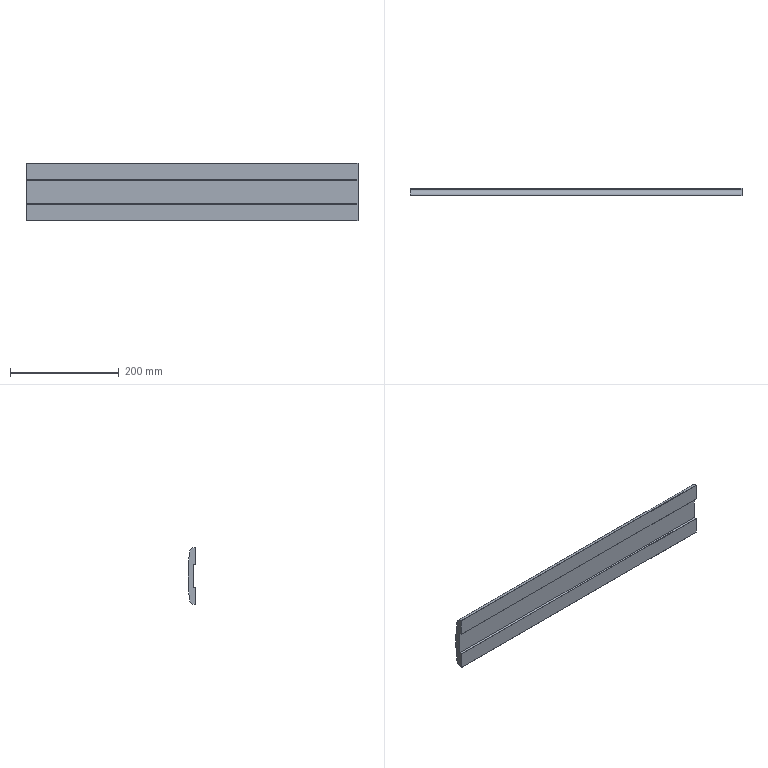Part | SolidWorks | features BaseBody 1 | 1 solid | 31 faces | box 611 x 14.5 x 106.047 mm | volume 703193 mm3 | cylinder 22 | plane 9 | commonest cylinder face diameters 0.2 x8 0.6 x6 22 x3 660 x3 0.4 x2
STEP:
#1=CARTESIAN_POINT('',(0.,60.288,-53.015));
#2=VERTEX_POINT('',#1);
#3=CARTESIAN_POINT('',(0.,60.72,-53.023));
#4=VERTEX_POINT('',#3);
#5=CARTESIAN_POINT('',(0.,60.72,-42.023));
#6=DIRECTION('',(1.,0.,0.));
#7=DIRECTION('',(0.,0.,-1.));
#8=AXIS2_PLACEMENT_3D('',#5,#6,#7);
#9=CIRCLE('',#8,11.);
#10=EDGE_CURVE('',#2,#4,#9,.T.);
#11=ORIENTED_EDGE('',*,*,#10,.T.);
#12=CARTESIAN_POINT('',(611.,60.72,-53.023));
#13=VERTEX_POINT('',#12);
#14=CARTESIAN_POINT('',(611.,60.72,-53.023));
#15=DIRECTION('',(1.,0.,0.));
#16=VECTOR('',#15,1000.);
#17=LINE('',#14,#16);
#18=EDGE_CURVE('',#4,#13,#17,.T.);
#19=ORIENTED_EDGE('',*,*,#18,.T.);
#20=CARTESIAN_POINT('',(611.,60.288,-53.015));
#21=VERTEX_POINT('',#20);
#22=CARTESIAN_POINT('',(611.,60.72,-42.023));
#23=DIRECTION('',(1.,0.,0.));
#24=DIRECTION('',(0.,0.,-1.));
#25=AXIS2_PLACEMENT_3D('',#22,#23,#24);
#26=CIRCLE('',#25,11.);
#27=EDGE_CURVE('',#21,#13,#26,.T.);
#28=ORIENTED_EDGE('',*,*,#27,.F.);
#29=CARTESIAN_POINT('',(611.,60.288,-53.015));
#30=DIRECTION('',(-1.,0.,0.));
#31=VECTOR('',#30,1000.);
#32=LINE('',#29,#31);
#33=EDGE_CURVE('',#21,#2,#32,.T.);
#34=ORIENTED_EDGE('',*,*,#33,.T.);
#35=EDGE_LOOP('',(#11,#19,#28,#34));
#36=FACE_OUTER_BOUND('',#35,.T.);
#37=CARTESIAN_POINT('',(611.,60.72,-42.023));
#38=DIRECTION('',(1.,0.,0.));
#39=DIRECTION('',(0.,0.,-1.));
#40=AXIS2_PLACEMENT_3D('',#37,#38,#39);
#41=CYLINDRICAL_SURFACE('',#40,11.);
#42=ADVANCED_FACE('',(#36),#41,.T.);
#43=CARTESIAN_POINT('',(611.,73.654,23.614));
#44=VERTEX_POINT('',#43);
#45=CARTESIAN_POINT('',(611.,73.654,-23.614));
#46=VERTEX_POINT('',#45);
#47=CARTESIAN_POINT('',(611.,-255.5,0.));
#48=DIRECTION('',(-1.,0.,0.));
#49=DIRECTION('',(0.,0.,-1.));
#50=AXIS2_PLACEMENT_3D('',#47,#48,#49);
#51=CIRCLE('',#50,330.);
#52=EDGE_CURVE('',#44,#46,#51,.T.);
#53=ORIENTED_EDGE('',*,*,#52,.T.);
#54=CARTESIAN_POINT('',(0.,73.654,-23.614));
#55=VERTEX_POINT('',#54);
#56=CARTESIAN_POINT('',(611.,73.654,-23.614));
#57=DIRECTION('',(-1.,0.,0.));
#58=VECTOR('',#57,1000.);
#59=LINE('',#56,#58);
#60=EDGE_CURVE('',#46,#55,#59,.T.);
#61=ORIENTED_EDGE('',*,*,#60,.T.);
#62=CARTESIAN_POINT('',(0.,73.654,23.614));
#63=VERTEX_POINT('',#62);
#64=CARTESIAN_POINT('',(0.,-255.5,0.));
#65=DIRECTION('',(1.,0.,0.));
#66=DIRECTION('',(0.,0.,-1.));
#67=AXIS2_PLACEMENT_3D('',#64,#65,#66);
#68=CIRCLE('',#67,330.);
#69=EDGE_CURVE('',#55,#63,#68,.T.);
#70=ORIENTED_EDGE('',*,*,#69,.T.);
#71=CARTESIAN_POINT('',(611.,73.654,23.614));
#72=DIRECTION('',(1.,0.,0.));
#73=VECTOR('',#72,1000.);
#74=LINE('',#71,#73);
#75=EDGE_CURVE('',#63,#44,#74,.T.);
#76=ORIENTED_EDGE('',*,*,#75,.T.);
#77=EDGE_LOOP('',(#53,#61,#70,#76));
#78=FACE_OUTER_BOUND('',#77,.T.);
#79=CARTESIAN_POINT('',(611.,-255.5,0.));
#80=DIRECTION('',(1.,0.,0.));
#81=DIRECTION('',(0.,0.,-1.));
#82=AXIS2_PLACEMENT_3D('',#79,#80,#81);
#83=CYLINDRICAL_SURFACE('',#82,330.);
#84=ADVANCED_FACE('',(#78),#83,.T.);
#85=CARTESIAN_POINT('',(611.,73.572,-23.705));
#86=VERTEX_POINT('',#85);
#87=CARTESIAN_POINT('',(611.,73.554,-23.607));
#88=DIRECTION('',(-1.,0.,0.));
#89=DIRECTION('',(0.,0.,-1.));
#90=AXIS2_PLACEMENT_3D('',#87,#88,#89);
#91=CIRCLE('',#90,0.1);
#92=EDGE_CURVE('',#46,#86,#91,.T.);
#93=ORIENTED_EDGE('',*,*,#92,.T.);
#94=CARTESIAN_POINT('',(0.,73.572,-23.705));
#95=VERTEX_POINT('',#94);
#96=CARTESIAN_POINT('',(611.,73.572,-23.705));
#97=DIRECTION('',(-1.,0.,0.));
#98=VECTOR('',#97,1000.);
#99=LINE('',#96,#98);
#100=EDGE_CURVE('',#86,#95,#99,.T.);
#101=ORIENTED_EDGE('',*,*,#100,.T.);
#102=CARTESIAN_POINT('',(0.,73.554,-23.607));
#103=DIRECTION('',(1.,0.,0.));
#104=DIRECTION('',(0.,0.,-1.));
#105=AXIS2_PLACEMENT_3D('',#102,#103,#104);
#106=CIRCLE('',#105,0.1);
#107=EDGE_CURVE('',#95,#55,#106,.T.);
#108=ORIENTED_EDGE('',*,*,#107,.T.);
#109=ORIENTED_EDGE('',*,*,#60,.F.);
#110=EDGE_LOOP('',(#93,#101,#108,#109));
#111=FACE_OUTER_BOUND('',#110,.T.);
#112=CARTESIAN_POINT('',(611.,73.554,-23.607));
#113=DIRECTION('',(1.,0.,0.));
#114=DIRECTION('',(0.,0.,-1.));
#115=AXIS2_PLACEMENT_3D('',#112,#113,#114);
#116=CYLINDRICAL_SURFACE('',#115,0.1);
#117=ADVANCED_FACE('',(#111),#116,.T.);
#118=CARTESIAN_POINT('',(611.,73.499,24.705));
#119=VERTEX_POINT('',#118);
#120=CARTESIAN_POINT('',(611.,73.455,25.284));
#121=VERTEX_POINT('',#120);
#122=CARTESIAN_POINT('',(611.,73.552,25.));
#123=DIRECTION('',(-1.,0.,0.));
#124=DIRECTION('',(0.,0.,-1.));
#125=AXIS2_PLACEMENT_3D('',#122,#123,#124);
#126=CIRCLE('',#125,0.3);
#127=EDGE_CURVE('',#119,#121,#126,.T.);
#128=ORIENTED_EDGE('',*,*,#127,.T.);
#129=CARTESIAN_POINT('',(611.,73.522,25.386));
#130=VERTEX_POINT('',#129);
#131=CARTESIAN_POINT('',(611.,73.422,25.378));
#132=DIRECTION('',(-1.,0.,0.));
#133=DIRECTION('',(0.,0.,-1.));
#134=AXIS2_PLACEMENT_3D('',#131,#132,#133);
#135=CIRCLE('',#134,0.1);
#136=EDGE_CURVE('',#130,#121,#135,.T.);
#137=ORIENTED_EDGE('',*,*,#136,.F.);
#138=CARTESIAN_POINT('',(611.,71.624,43.473));
#139=VERTEX_POINT('',#138);
#140=CARTESIAN_POINT('',(611.,-255.5,0.002391));
#141=DIRECTION('',(1.,0.,0.));
#142=DIRECTION('',(0.,0.,-1.));
#143=AXIS2_PLACEMENT_3D('',#140,#141,#142);
#144=CIRCLE('',#143,330.);
#145=EDGE_CURVE('',#130,#139,#144,.T.);
#146=ORIENTED_EDGE('',*,*,#145,.T.);
#147=CARTESIAN_POINT('',(611.,60.288,53.015));
#148=VERTEX_POINT('',#147);
#149=CARTESIAN_POINT('',(611.,60.72,42.023));
#150=DIRECTION('',(1.,0.,0.));
#151=DIRECTION('',(0.,0.,-1.));
#152=AXIS2_PLACEMENT_3D('',#149,#150,#151);
#153=CIRCLE('',#152,11.);
#154=EDGE_CURVE('',#139,#148,#153,.T.);
#155=ORIENTED_EDGE('',*,*,#154,.T.);
#156=CARTESIAN_POINT('',(611.,60.,52.715));
#157=VERTEX_POINT('',#156);
#158=CARTESIAN_POINT('',(611.,60.3,52.715));
#159=DIRECTION('',(-1.,0.,0.));
#160=DIRECTION('',(0.,0.,-1.));
#161=AXIS2_PLACEMENT_3D('',#158,#159,#160);
#162=CIRCLE('',#161,0.3);
#163=EDGE_CURVE('',#157,#148,#162,.T.);
#164=ORIENTED_EDGE('',*,*,#163,.F.);
#165=CARTESIAN_POINT('',(611.,60.,22.2));
#166=VERTEX_POINT('',#165);
#167=CARTESIAN_POINT('',(611.,60.,0.002391));
#168=DIRECTION('',(0.,0.,-1.));
#169=VECTOR('',#168,1000.);
#170=LINE('',#167,#169);
#171=EDGE_CURVE('',#157,#166,#170,.T.);
#172=ORIENTED_EDGE('',*,*,#171,.T.);
#173=CARTESIAN_POINT('',(611.,60.2,22.));
#174=VERTEX_POINT('',#173);
#175=CARTESIAN_POINT('',(611.,60.2,22.2));
#176=DIRECTION('',(-1.,0.,0.));
#177=DIRECTION('',(0.,0.,-1.));
#178=AXIS2_PLACEMENT_3D('',#175,#176,#177);
#179=CIRCLE('',#178,0.2);
#180=EDGE_CURVE('',#174,#166,#179,.T.);
#181=ORIENTED_EDGE('',*,*,#180,.F.);
#182=CARTESIAN_POINT('',(611.,64.5,22.));
#183=VERTEX_POINT('',#182);
#184=CARTESIAN_POINT('',(611.,-255.5,22.));
#185=DIRECTION('',(0.,1.,0.));
#186=VECTOR('',#185,1000.);
#187=LINE('',#184,#186);
#188=EDGE_CURVE('',#174,#183,#187,.T.);
#189=ORIENTED_EDGE('',*,*,#188,.T.);
#190=CARTESIAN_POINT('',(611.,64.5,-22.));
#191=VERTEX_POINT('',#190);
#192=CARTESIAN_POINT('',(611.,64.5,0.002391));
#193=DIRECTION('',(0.,0.,-1.));
#194=VECTOR('',#193,1000.);
#195=LINE('',#192,#194);
#196=EDGE_CURVE('',#183,#191,#195,.T.);
#197=ORIENTED_EDGE('',*,*,#196,.T.);
#198=CARTESIAN_POINT('',(611.,60.2,-22.));
#199=VERTEX_POINT('',#198);
#200=CARTESIAN_POINT('',(611.,-255.5,-22.));
#201=DIRECTION('',(0.,-1.,0.));
#202=VECTOR('',#201,1000.);
#203=LINE('',#200,#202);
#204=EDGE_CURVE('',#191,#199,#203,.T.);
#205=ORIENTED_EDGE('',*,*,#204,.T.);
#206=CARTESIAN_POINT('',(611.,60.,-22.2));
#207=VERTEX_POINT('',#206);
#208=CARTESIAN_POINT('',(611.,60.2,-22.2));
#209=DIRECTION('',(-1.,0.,0.));
#210=DIRECTION('',(0.,0.,-1.));
#211=AXIS2_PLACEMENT_3D('',#208,#209,#210);
#212=CIRCLE('',#211,0.2);
#213=EDGE_CURVE('',#207,#199,#212,.T.);
#214=ORIENTED_EDGE('',*,*,#213,.F.);
#215=CARTESIAN_POINT('',(611.,60.,-52.715));
#216=VERTEX_POINT('',#215);
#217=CARTESIAN_POINT('',(611.,60.,0.002391));
#218=DIRECTION('',(0.,0.,-1.));
#219=VECTOR('',#218,1000.);
#220=LINE('',#217,#219);
#221=EDGE_CURVE('',#207,#216,#220,.T.);
#222=ORIENTED_EDGE('',*,*,#221,.T.);
#223=CARTESIAN_POINT('',(611.,60.3,-52.715));
#224=DIRECTION('',(-1.,0.,0.));
#225=DIRECTION('',(0.,0.,-1.));
#226=AXIS2_PLACEMENT_3D('',#223,#224,#225);
#227=CIRCLE('',#226,0.3);
#228=EDGE_CURVE('',#21,#216,#227,.T.);
#229=ORIENTED_EDGE('',*,*,#228,.F.);
#230=ORIENTED_EDGE('',*,*,#27,.T.);
#231=CARTESIAN_POINT('',(611.,71.624,-43.473));
#232=VERTEX_POINT('',#231);
#233=CARTESIAN_POINT('',(611.,60.72,-42.023));
#234=DIRECTION('',(1.,0.,0.));
#235=DIRECTION('',(0.,0.,-1.));
#236=AXIS2_PLACEMENT_3D('',#233,#234,#235);
#237=CIRCLE('',#236,11.);
#238=EDGE_CURVE('',#13,#232,#237,.T.);
#239=ORIENTED_EDGE('',*,*,#238,.T.);
#240=CARTESIAN_POINT('',(611.,73.522,-25.386));
#241=VERTEX_POINT('',#240);
#242=CARTESIAN_POINT('',(611.,-255.5,-0.002391));
#243=DIRECTION('',(1.,0.,0.));
#244=DIRECTION('',(0.,0.,-1.));
#245=AXIS2_PLACEMENT_3D('',#242,#243,#244);
#246=CIRCLE('',#245,330.);
#247=EDGE_CURVE('',#232,#241,#246,.T.);
#248=ORIENTED_EDGE('',*,*,#247,.T.);
#249=CARTESIAN_POINT('',(611.,73.455,-25.284));
#250=VERTEX_POINT('',#249);
#251=CARTESIAN_POINT('',(611.,73.422,-25.378));
#252=DIRECTION('',(-1.,0.,0.));
#253=DIRECTION('',(0.,0.,-1.));
#254=AXIS2_PLACEMENT_3D('',#251,#252,#253);
#255=CIRCLE('',#254,0.1);
#256=EDGE_CURVE('',#250,#241,#255,.T.);
#257=ORIENTED_EDGE('',*,*,#256,.F.);
#258=CARTESIAN_POINT('',(611.,73.499,-24.705));
#259=VERTEX_POINT('',#258);
#260=CARTESIAN_POINT('',(611.,73.552,-25.));
#261=DIRECTION('',(-1.,0.,0.));
#262=DIRECTION('',(0.,0.,-1.));
#263=AXIS2_PLACEMENT_3D('',#260,#261,#262);
#264=CIRCLE('',#263,0.3);
#265=EDGE_CURVE('',#250,#259,#264,.T.);
#266=ORIENTED_EDGE('',*,*,#265,.T.);
#267=CARTESIAN_POINT('',(611.,73.581,-24.614));
#268=VERTEX_POINT('',#267);
#269=CARTESIAN_POINT('',(611.,73.481,-24.607));
#270=DIRECTION('',(-1.,0.,0.));
#271=DIRECTION('',(0.,0.,-1.));
#272=AXIS2_PLACEMENT_3D('',#269,#270,#271);
#273=CIRCLE('',#272,0.1);
#274=EDGE_CURVE('',#268,#259,#273,.T.);
#275=ORIENTED_EDGE('',*,*,#274,.F.);
#276=CARTESIAN_POINT('',(611.,73.598,-24.386));
#277=VERTEX_POINT('',#276);
#278=CARTESIAN_POINT('',(611.,73.581,-24.614));
#279=DIRECTION('',(0.,0.07436,0.9972));
#280=VECTOR('',#279,1000.);
#281=LINE('',#278,#280);
#282=EDGE_CURVE('',#268,#277,#281,.T.);
#283=ORIENTED_EDGE('',*,*,#282,.T.);
#284=CARTESIAN_POINT('',(611.,73.53,-24.284));
#285=VERTEX_POINT('',#284);
#286=CARTESIAN_POINT('',(611.,73.498,-24.379));
#287=DIRECTION('',(-1.,0.,0.));
#288=DIRECTION('',(0.,0.,-1.));
#289=AXIS2_PLACEMENT_3D('',#286,#287,#288);
#290=CIRCLE('',#289,0.1);
#291=EDGE_CURVE('',#285,#277,#290,.T.);
#292=ORIENTED_EDGE('',*,*,#291,.F.);
#293=CARTESIAN_POINT('',(611.,73.627,-24.));
#294=DIRECTION('',(-1.,0.,0.));
#295=DIRECTION('',(0.,0.,-1.));
#296=AXIS2_PLACEMENT_3D('',#293,#294,#295);
#297=CIRCLE('',#296,0.3);
#298=EDGE_CURVE('',#285,#86,#297,.T.);
#299=ORIENTED_EDGE('',*,*,#298,.T.);
#300=ORIENTED_EDGE('',*,*,#92,.F.);
#301=ORIENTED_EDGE('',*,*,#52,.F.);
#302=CARTESIAN_POINT('',(611.,73.572,23.705));
#303=VERTEX_POINT('',#302);
#304=CARTESIAN_POINT('',(611.,73.554,23.607));
#305=DIRECTION('',(1.,0.,0.));
#306=DIRECTION('',(0.,0.,-1.));
#307=AXIS2_PLACEMENT_3D('',#304,#305,#306);
#308=CIRCLE('',#307,0.1);
#309=EDGE_CURVE('',#44,#303,#308,.T.);
#310=ORIENTED_EDGE('',*,*,#309,.T.);
#311=CARTESIAN_POINT('',(611.,73.53,24.284));
#312=VERTEX_POINT('',#311);
#313=CARTESIAN_POINT('',(611.,73.627,24.));
#314=DIRECTION('',(-1.,0.,0.));
#315=DIRECTION('',(0.,0.,-1.));
#316=AXIS2_PLACEMENT_3D('',#313,#314,#315);
#317=CIRCLE('',#316,0.3);
#318=EDGE_CURVE('',#303,#312,#317,.T.);
#319=ORIENTED_EDGE('',*,*,#318,.T.);
#320=CARTESIAN_POINT('',(611.,73.598,24.386));
#321=VERTEX_POINT('',#320);
#322=CARTESIAN_POINT('',(611.,73.498,24.379));
#323=DIRECTION('',(-1.,0.,0.));
#324=DIRECTION('',(0.,0.,-1.));
#325=AXIS2_PLACEMENT_3D('',#322,#323,#324);
#326=CIRCLE('',#325,0.1);
#327=EDGE_CURVE('',#321,#312,#326,.T.);
#328=ORIENTED_EDGE('',*,*,#327,.F.);
#329=CARTESIAN_POINT('',(611.,73.581,24.614));
#330=VERTEX_POINT('',#329);
#331=CARTESIAN_POINT('',(611.,73.598,24.386));
#332=DIRECTION('',(0.,-0.07436,0.9972));
#333=VECTOR('',#332,1000.);
#334=LINE('',#331,#333);
#335=EDGE_CURVE('',#321,#330,#334,.T.);
#336=ORIENTED_EDGE('',*,*,#335,.T.);
#337=CARTESIAN_POINT('',(611.,73.481,24.607));
#338=DIRECTION('',(-1.,0.,0.));
#339=DIRECTION('',(0.,0.,-1.));
#340=AXIS2_PLACEMENT_3D('',#337,#338,#339);
#341=CIRCLE('',#340,0.1);
#342=EDGE_CURVE('',#119,#330,#341,.T.);
#343=ORIENTED_EDGE('',*,*,#342,.F.);
#344=EDGE_LOOP('',(#128,#137,#146,#155,#164,#172,#181,#189,#197,#205,#214,#222,#229,#230,#239,#248,#257,#266,#275,#283,#292,#299,#300,#301,#310,#319,#328,#336,#343));
#345=FACE_OUTER_BOUND('',#344,.T.);
#346=CARTESIAN_POINT('',(611.,-255.5,0.002391));
#347=DIRECTION('',(1.,0.,0.));
#348=DIRECTION('',(0.,0.,-1.));
#349=AXIS2_PLACEMENT_3D('',#346,#347,#348);
#350=PLANE('',#349);
#351=ADVANCED_FACE('',(#345),#350,.T.);
#352=ORIENTED_EDGE('',*,*,#309,.F.);
#353=ORIENTED_EDGE('',*,*,#75,.F.);
#354=CARTESIAN_POINT('',(0.,73.572,23.705));
#355=VERTEX_POINT('',#354);
#356=CARTESIAN_POINT('',(0.,73.554,23.607));
#357=DIRECTION('',(1.,0.,0.));
#358=DIRECTION('',(0.,0.,-1.));
#359=AXIS2_PLACEMENT_3D('',#356,#357,#358);
#360=CIRCLE('',#359,0.1);
#361=EDGE_CURVE('',#63,#355,#360,.T.);
#362=ORIENTED_EDGE('',*,*,#361,.T.);
#363=CARTESIAN_POINT('',(611.,73.572,23.705));
#364=DIRECTION('',(1.,0.,0.));
#365=VECTOR('',#364,1000.);
#366=LINE('',#363,#365);
#367=EDGE_CURVE('',#355,#303,#366,.T.);
#368=ORIENTED_EDGE('',*,*,#367,.T.);
#369=EDGE_LOOP('',(#352,#353,#362,#368));
#370=FACE_OUTER_BOUND('',#369,.T.);
#371=CARTESIAN_POINT('',(611.,73.554,23.607));
#372=DIRECTION('',(1.,0.,0.));
#373=DIRECTION('',(0.,0.,-1.));
#374=AXIS2_PLACEMENT_3D('',#371,#372,#373);
#375=CYLINDRICAL_SURFACE('',#374,0.1);
#376=ADVANCED_FACE('',(#370),#375,.T.);
#377=CARTESIAN_POINT('',(0.,73.455,25.284));
#378=VERTEX_POINT('',#377);
#379=CARTESIAN_POINT('',(0.,73.522,25.386));
#380=VERTEX_POINT('',#379);
#381=CARTESIAN_POINT('',(0.,73.422,25.378));
#382=DIRECTION('',(1.,0.,0.));
#383=DIRECTION('',(0.,0.,-1.));
#384=AXIS2_PLACEMENT_3D('',#381,#382,#383);
#385=CIRCLE('',#384,0.1);
#386=EDGE_CURVE('',#378,#380,#385,.T.);
#387=ORIENTED_EDGE('',*,*,#386,.F.);
#388=CARTESIAN_POINT('',(0.,73.499,24.705));
#389=VERTEX_POINT('',#388);
#390=CARTESIAN_POINT('',(0.,73.552,25.));
#391=DIRECTION('',(1.,0.,0.));
#392=DIRECTION('',(0.,0.,-1.));
#393=AXIS2_PLACEMENT_3D('',#390,#391,#392);
#394=CIRCLE('',#393,0.3);
#395=EDGE_CURVE('',#378,#389,#394,.T.);
#396=ORIENTED_EDGE('',*,*,#395,.T.);
#397=CARTESIAN_POINT('',(0.,73.581,24.614));
#398=VERTEX_POINT('',#397);
#399=CARTESIAN_POINT('',(0.,73.481,24.607));
#400=DIRECTION('',(1.,0.,0.));
#401=DIRECTION('',(0.,0.,-1.));
#402=AXIS2_PLACEMENT_3D('',#399,#400,#401);
#403=CIRCLE('',#402,0.1);
#404=EDGE_CURVE('',#398,#389,#403,.T.);
#405=ORIENTED_EDGE('',*,*,#404,.F.);
#406=CARTESIAN_POINT('',(0.,73.598,24.386));
#407=VERTEX_POINT('',#406);
#408=CARTESIAN_POINT('',(0.,73.598,24.386));
#409=DIRECTION('',(0.,0.07436,-0.9972));
#410=VECTOR('',#409,1000.);
#411=LINE('',#408,#410);
#412=EDGE_CURVE('',#398,#407,#411,.T.);
#413=ORIENTED_EDGE('',*,*,#412,.T.);
#414=CARTESIAN_POINT('',(0.,73.53,24.284));
#415=VERTEX_POINT('',#414);
#416=CARTESIAN_POINT('',(0.,73.498,24.379));
#417=DIRECTION('',(1.,0.,0.));
#418=DIRECTION('',(0.,0.,-1.));
#419=AXIS2_PLACEMENT_3D('',#416,#417,#418);
#420=CIRCLE('',#419,0.1);
#421=EDGE_CURVE('',#415,#407,#420,.T.);
#422=ORIENTED_EDGE('',*,*,#421,.F.);
#423=CARTESIAN_POINT('',(0.,73.627,24.));
#424=DIRECTION('',(-1.,0.,0.));
#425=DIRECTION('',(0.,0.,-1.));
#426=AXIS2_PLACEMENT_3D('',#423,#424,#425);
#427=CIRCLE('',#426,0.3);
#428=EDGE_CURVE('',#355,#415,#427,.T.);
#429=ORIENTED_EDGE('',*,*,#428,.F.);
#430=ORIENTED_EDGE('',*,*,#361,.F.);
#431=ORIENTED_EDGE('',*,*,#69,.F.);
#432=ORIENTED_EDGE('',*,*,#107,.F.);
#433=CARTESIAN_POINT('',(0.,73.53,-24.284));
#434=VERTEX_POINT('',#433);
#435=CARTESIAN_POINT('',(0.,73.627,-24.));
#436=DIRECTION('',(-1.,0.,0.));
#437=DIRECTION('',(0.,0.,-1.));
#438=AXIS2_PLACEMENT_3D('',#435,#436,#437);
#439=CIRCLE('',#438,0.3);
#440=EDGE_CURVE('',#434,#95,#439,.T.);
#441=ORIENTED_EDGE('',*,*,#440,.F.);
#442=CARTESIAN_POINT('',(0.,73.598,-24.386));
#443=VERTEX_POINT('',#442);
#444=CARTESIAN_POINT('',(0.,73.498,-24.379));
#445=DIRECTION('',(1.,0.,0.));
#446=DIRECTION('',(0.,0.,-1.));
#447=AXIS2_PLACEMENT_3D('',#444,#445,#446);
#448=CIRCLE('',#447,0.1);
#449=EDGE_CURVE('',#443,#434,#448,.T.);
#450=ORIENTED_EDGE('',*,*,#449,.F.);
#451=CARTESIAN_POINT('',(0.,73.581,-24.614));
#452=VERTEX_POINT('',#451);
#453=CARTESIAN_POINT('',(0.,73.581,-24.614));
#454=DIRECTION('',(0.,-0.07436,-0.9972));
#455=VECTOR('',#454,1000.);
#456=LINE('',#453,#455);
#457=EDGE_CURVE('',#443,#452,#456,.T.);
#458=ORIENTED_EDGE('',*,*,#457,.T.);
#459=CARTESIAN_POINT('',(0.,73.499,-24.705));
#460=VERTEX_POINT('',#459);
#461=CARTESIAN_POINT('',(0.,73.481,-24.607));
#462=DIRECTION('',(1.,0.,0.));
#463=DIRECTION('',(0.,0.,-1.));
#464=AXIS2_PLACEMENT_3D('',#461,#462,#463);
#465=CIRCLE('',#464,0.1);
#466=EDGE_CURVE('',#460,#452,#465,.T.);
#467=ORIENTED_EDGE('',*,*,#466,.F.);
#468=CARTESIAN_POINT('',(0.,73.455,-25.284));
#469=VERTEX_POINT('',#468);
#470=CARTESIAN_POINT('',(0.,73.552,-25.));
#471=DIRECTION('',(1.,0.,0.));
#472=DIRECTION('',(0.,0.,-1.));
#473=AXIS2_PLACEMENT_3D('',#470,#471,#472);
#474=CIRCLE('',#473,0.3);
#475=EDGE_CURVE('',#460,#469,#474,.T.);
#476=ORIENTED_EDGE('',*,*,#475,.T.);
#477=CARTESIAN_POINT('',(0.,73.522,-25.386));
#478=VERTEX_POINT('',#477);
#479=CARTESIAN_POINT('',(0.,73.422,-25.378));
#480=DIRECTION('',(1.,0.,0.));
#481=DIRECTION('',(0.,0.,-1.));
#482=AXIS2_PLACEMENT_3D('',#479,#480,#481);
#483=CIRCLE('',#482,0.1);
#484=EDGE_CURVE('',#478,#469,#483,.T.);
#485=ORIENTED_EDGE('',*,*,#484,.F.);
#486=CARTESIAN_POINT('',(0.,71.624,-43.473));
#487=VERTEX_POINT('',#486);
#488=CARTESIAN_POINT('',(0.,-255.5,-0.002391));
#489=DIRECTION('',(1.,0.,0.));
#490=DIRECTION('',(0.,0.,-1.));
#491=AXIS2_PLACEMENT_3D('',#488,#489,#490);
#492=CIRCLE('',#491,330.);
#493=EDGE_CURVE('',#487,#478,#492,.T.);
#494=ORIENTED_EDGE('',*,*,#493,.F.);
#495=CARTESIAN_POINT('',(0.,60.72,-42.023));
#496=DIRECTION('',(1.,0.,0.));
#497=DIRECTION('',(0.,0.,-1.));
#498=AXIS2_PLACEMENT_3D('',#495,#496,#497);
#499=CIRCLE('',#498,11.);
#500=EDGE_CURVE('',#4,#487,#499,.T.);
#501=ORIENTED_EDGE('',*,*,#500,.F.);
#502=ORIENTED_EDGE('',*,*,#10,.F.);
#503=CARTESIAN_POINT('',(0.,60.,-52.715));
#504=VERTEX_POINT('',#503);
#505=CARTESIAN_POINT('',(0.,60.3,-52.715));
#506=DIRECTION('',(1.,0.,0.));
#507=DIRECTION('',(0.,0.,-1.));
#508=AXIS2_PLACEMENT_3D('',#505,#506,#507);
#509=CIRCLE('',#508,0.3);
#510=EDGE_CURVE('',#504,#2,#509,.T.);
#511=ORIENTED_EDGE('',*,*,#510,.F.);
#512=CARTESIAN_POINT('',(0.,60.,-22.2));
#513=VERTEX_POINT('',#512);
#514=CARTESIAN_POINT('',(0.,60.,0.002391));
#515=DIRECTION('',(0.,0.,-1.));
#516=VECTOR('',#515,1000.);
#517=LINE('',#514,#516);
#518=EDGE_CURVE('',#513,#504,#517,.T.);
#519=ORIENTED_EDGE('',*,*,#518,.F.);
#520=CARTESIAN_POINT('',(0.,60.2,-22.));
#521=VERTEX_POINT('',#520);
#522=CARTESIAN_POINT('',(0.,60.2,-22.2));
#523=DIRECTION('',(1.,0.,0.));
#524=DIRECTION('',(0.,0.,-1.));
#525=AXIS2_PLACEMENT_3D('',#522,#523,#524);
#526=CIRCLE('',#525,0.2);
#527=EDGE_CURVE('',#521,#513,#526,.T.);
#528=ORIENTED_EDGE('',*,*,#527,.F.);
#529=CARTESIAN_POINT('',(0.,64.5,-22.));
#530=VERTEX_POINT('',#529);
#531=CARTESIAN_POINT('',(0.,-255.5,-22.));
#532=DIRECTION('',(0.,-1.,0.));
#533=VECTOR('',#532,1000.);
#534=LINE('',#531,#533);
#535=EDGE_CURVE('',#530,#521,#534,.T.);
#536=ORIENTED_EDGE('',*,*,#535,.F.);
#537=CARTESIAN_POINT('',(0.,64.5,22.));
#538=VERTEX_POINT('',#537);
#539=CARTESIAN_POINT('',(0.,64.5,0.002391));
#540=DIRECTION('',(0.,0.,-1.));
#541=VECTOR('',#540,1000.);
#542=LINE('',#539,#541);
#543=EDGE_CURVE('',#538,#530,#542,.T.);
#544=ORIENTED_EDGE('',*,*,#543,.F.);
#545=CARTESIAN_POINT('',(0.,60.2,22.));
#546=VERTEX_POINT('',#545);
#547=CARTESIAN_POINT('',(0.,-255.5,22.));
#548=DIRECTION('',(0.,1.,0.));
#549=VECTOR('',#548,1000.);
#550=LINE('',#547,#549);
#551=EDGE_CURVE('',#546,#538,#550,.T.);
#552=ORIENTED_EDGE('',*,*,#551,.F.);
#553=CARTESIAN_POINT('',(0.,60.,22.2));
#554=VERTEX_POINT('',#553);
#555=CARTESIAN_POINT('',(0.,60.2,22.2));
#556=DIRECTION('',(1.,0.,0.));
#557=DIRECTION('',(0.,0.,-1.));
#558=AXIS2_PLACEMENT_3D('',#555,#556,#557);
#559=CIRCLE('',#558,0.2);
#560=EDGE_CURVE('',#554,#546,#559,.T.);
#561=ORIENTED_EDGE('',*,*,#560,.F.);
#562=CARTESIAN_POINT('',(0.,60.,52.715));
#563=VERTEX_POINT('',#562);
#564=CARTESIAN_POINT('',(0.,60.,0.002391));
#565=DIRECTION('',(0.,0.,-1.));
#566=VECTOR('',#565,1000.);
#567=LINE('',#564,#566);
#568=EDGE_CURVE('',#563,#554,#567,.T.);
#569=ORIENTED_EDGE('',*,*,#568,.F.);
#570=CARTESIAN_POINT('',(0.,60.288,53.015));
#571=VERTEX_POINT('',#570);
#572=CARTESIAN_POINT('',(0.,60.3,52.715));
#573=DIRECTION('',(1.,0.,0.));
#574=DIRECTION('',(0.,0.,-1.));
#575=AXIS2_PLACEMENT_3D('',#572,#573,#574);
#576=CIRCLE('',#575,0.3);
#577=EDGE_CURVE('',#571,#563,#576,.T.);
#578=ORIENTED_EDGE('',*,*,#577,.F.);
#579=CARTESIAN_POINT('',(0.,71.624,43.473));
#580=VERTEX_POINT('',#579);
#581=CARTESIAN_POINT('',(0.,60.72,42.023));
#582=DIRECTION('',(1.,0.,0.));
#583=DIRECTION('',(0.,0.,-1.));
#584=AXIS2_PLACEMENT_3D('',#581,#582,#583);
#585=CIRCLE('',#584,11.);
#586=EDGE_CURVE('',#580,#571,#585,.T.);
#587=ORIENTED_EDGE('',*,*,#586,.F.);
#588=CARTESIAN_POINT('',(0.,-255.5,0.002391));
#589=DIRECTION('',(1.,0.,0.));
#590=DIRECTION('',(0.,0.,-1.));
#591=AXIS2_PLACEMENT_3D('',#588,#589,#590);
#592=CIRCLE('',#591,330.);
#593=EDGE_CURVE('',#380,#580,#592,.T.);
#594=ORIENTED_EDGE('',*,*,#593,.F.);
#595=EDGE_LOOP('',(#387,#396,#405,#413,#422,#429,#430,#431,#432,#441,#450,#458,#467,#476,#485,#494,#501,#502,#511,#519,#528,#536,#544,#552,#561,#569,#578,#587,#594));
#596=FACE_OUTER_BOUND('',#595,.T.);
#597=CARTESIAN_POINT('',(0.,-255.5,0.002391));
#598=DIRECTION('',(1.,0.,0.));
#599=DIRECTION('',(0.,0.,-1.));
#600=AXIS2_PLACEMENT_3D('',#597,#598,#599);
#601=PLANE('',#600);
#602=ADVANCED_FACE('',(#596),#601,.F.);
#603=ORIENTED_EDGE('',*,*,#100,.F.);
#604=ORIENTED_EDGE('',*,*,#298,.F.);
#605=CARTESIAN_POINT('',(611.,73.53,-24.284));
#606=DIRECTION('',(1.,0.,0.));
#607=VECTOR('',#606,1000.);
#608=LINE('',#605,#607);
#609=EDGE_CURVE('',#434,#285,#608,.T.);
#610=ORIENTED_EDGE('',*,*,#609,.F.);
#611=ORIENTED_EDGE('',*,*,#440,.T.);
#612=EDGE_LOOP('',(#603,#604,#610,#611));
#613=FACE_OUTER_BOUND('',#612,.T.);
#614=CARTESIAN_POINT('',(611.,73.627,-24.));
#615=DIRECTION('',(1.,0.,0.));
#616=DIRECTION('',(0.,0.,-1.));
#617=AXIS2_PLACEMENT_3D('',#614,#615,#616);
#618=CYLINDRICAL_SURFACE('',#617,0.3);
#619=ADVANCED_FACE('',(#613),#618,.F.);
#620=ORIENTED_EDGE('',*,*,#247,.F.);
#621=CARTESIAN_POINT('',(611.,71.624,-43.473));
#622=DIRECTION('',(-1.,0.,0.));
#623=VECTOR('',#622,1000.);
#624=LINE('',#621,#623);
#625=EDGE_CURVE('',#232,#487,#624,.T.);
#626=ORIENTED_EDGE('',*,*,#625,.T.);
#627=ORIENTED_EDGE('',*,*,#493,.T.);
#628=CARTESIAN_POINT('',(611.,73.522,-25.386));
#629=DIRECTION('',(1.,0.,0.));
#630=VECTOR('',#629,1000.);
#631=LINE('',#628,#630);
#632=EDGE_CURVE('',#478,#241,#631,.T.);
#633=ORIENTED_EDGE('',*,*,#632,.T.);
#634=EDGE_LOOP('',(#620,#626,#627,#633));
#635=FACE_OUTER_BOUND('',#634,.T.);
#636=CARTESIAN_POINT('',(611.,-255.5,-0.002391));
#637=DIRECTION('',(1.,0.,0.));
#638=DIRECTION('',(0.,0.,-1.));
#639=AXIS2_PLACEMENT_3D('',#636,#637,#638);
#640=CYLINDRICAL_SURFACE('',#639,330.);
#641=ADVANCED_FACE('',(#635),#640,.T.);
#642=ORIENTED_EDGE('',*,*,#18,.F.);
#643=ORIENTED_EDGE('',*,*,#500,.T.);
#644=ORIENTED_EDGE('',*,*,#625,.F.);
#645=ORIENTED_EDGE('',*,*,#238,.F.);
#646=EDGE_LOOP('',(#642,#643,#644,#645));
#647=FACE_OUTER_BOUND('',#646,.T.);
#648=CARTESIAN_POINT('',(611.,60.72,-42.023));
#649=DIRECTION('',(1.,0.,0.));
#650=DIRECTION('',(0.,0.,-1.));
#651=AXIS2_PLACEMENT_3D('',#648,#649,#650);
#652=CYLINDRICAL_SURFACE('',#651,11.);
#653=ADVANCED_FACE('',(#647),#652,.T.);
#654=CARTESIAN_POINT('',(611.,60.,-52.715));
#655=DIRECTION('',(-1.,0.,0.));
#656=VECTOR('',#655,1000.);
#657=LINE('',#654,#656);
#658=EDGE_CURVE('',#216,#504,#657,.T.);
#659=ORIENTED_EDGE('',*,*,#658,.F.);
#660=ORIENTED_EDGE('',*,*,#221,.F.);
#661=CARTESIAN_POINT('',(611.,60.,-22.2));
#662=DIRECTION('',(1.,0.,0.));
#663=VECTOR('',#662,1000.);
#664=LINE('',#661,#663);
#665=EDGE_CURVE('',#513,#207,#664,.T.);
#666=ORIENTED_EDGE('',*,*,#665,.F.);
#667=ORIENTED_EDGE('',*,*,#518,.T.);
#668=EDGE_LOOP('',(#659,#660,#666,#667));
#669=FACE_OUTER_BOUND('',#668,.T.);
#670=CARTESIAN_POINT('',(611.,60.,-22.2));
#671=DIRECTION('',(0.,1.,0.));
#672=DIRECTION('',(0.,0.,1.));
#673=AXIS2_PLACEMENT_3D('',#670,#671,#672);
#674=PLANE('',#673);
#675=ADVANCED_FACE('',(#669),#674,.F.);
#676=CARTESIAN_POINT('',(611.,60.2,-22.));
#677=DIRECTION('',(-1.,0.,0.));
#678=VECTOR('',#677,1000.);
#679=LINE('',#676,#678);
#680=EDGE_CURVE('',#199,#521,#679,.T.);
#681=ORIENTED_EDGE('',*,*,#680,.F.);
#682=ORIENTED_EDGE('',*,*,#204,.F.);
#683=CARTESIAN_POINT('',(611.,64.5,-22.));
#684=DIRECTION('',(1.,0.,0.));
#685=VECTOR('',#684,1000.);
#686=LINE('',#683,#685);
#687=EDGE_CURVE('',#530,#191,#686,.T.);
#688=ORIENTED_EDGE('',*,*,#687,.F.);
#689=ORIENTED_EDGE('',*,*,#535,.T.);
#690=EDGE_LOOP('',(#681,#682,#688,#689));
#691=FACE_OUTER_BOUND('',#690,.T.);
#692=CARTESIAN_POINT('',(611.,64.5,-22.));
#693=DIRECTION('',(0.,0.,-1.));
#694=DIRECTION('',(-1.,0.,0.));
#695=AXIS2_PLACEMENT_3D('',#692,#693,#694);
#696=PLANE('',#695);
#697=ADVANCED_FACE('',(#691),#696,.F.);
#698=ORIENTED_EDGE('',*,*,#687,.T.);
#699=ORIENTED_EDGE('',*,*,#196,.F.);
#700=CARTESIAN_POINT('',(611.,64.5,22.));
#701=DIRECTION('',(1.,0.,0.));
#702=VECTOR('',#701,1000.);
#703=LINE('',#700,#702);
#704=EDGE_CURVE('',#538,#183,#703,.T.);
#705=ORIENTED_EDGE('',*,*,#704,.F.);
#706=ORIENTED_EDGE('',*,*,#543,.T.);
#707=EDGE_LOOP('',(#698,#699,#705,#706));
#708=FACE_OUTER_BOUND('',#707,.T.);
#709=CARTESIAN_POINT('',(611.,64.5,22.));
#710=DIRECTION('',(0.,1.,0.));
#711=DIRECTION('',(0.,0.,1.));
#712=AXIS2_PLACEMENT_3D('',#709,#710,#711);
#713=PLANE('',#712);
#714=ADVANCED_FACE('',(#708),#713,.F.);
#715=ORIENTED_EDGE('',*,*,#704,.T.);
#716=ORIENTED_EDGE('',*,*,#188,.F.);
#717=CARTESIAN_POINT('',(611.,60.2,22.));
#718=DIRECTION('',(1.,0.,0.));
#719=VECTOR('',#718,1000.);
#720=LINE('',#717,#719);
#721=EDGE_CURVE('',#546,#174,#720,.T.);
#722=ORIENTED_EDGE('',*,*,#721,.F.);
#723=ORIENTED_EDGE('',*,*,#551,.T.);
#724=EDGE_LOOP('',(#715,#716,#722,#723));
#725=FACE_OUTER_BOUND('',#724,.T.);
#726=CARTESIAN_POINT('',(611.,60.2,22.));
#727=DIRECTION('',(0.,0.,1.));
#728=DIRECTION('',(1.,0.,0.));
#729=AXIS2_PLACEMENT_3D('',#726,#727,#728);
#730=PLANE('',#729);
#731=ADVANCED_FACE('',(#725),#730,.F.);
#732=CARTESIAN_POINT('',(611.,60.,22.2));
#733=DIRECTION('',(-1.,0.,0.));
#734=VECTOR('',#733,1000.);
#735=LINE('',#732,#734);
#736=EDGE_CURVE('',#166,#554,#735,.T.);
#737=ORIENTED_EDGE('',*,*,#736,.F.);
#738=ORIENTED_EDGE('',*,*,#171,.F.);
#739=CARTESIAN_POINT('',(611.,60.,52.715));
#740=DIRECTION('',(1.,0.,0.));
#741=VECTOR('',#740,1000.);
#742=LINE('',#739,#741);
#743=EDGE_CURVE('',#563,#157,#742,.T.);
#744=ORIENTED_EDGE('',*,*,#743,.F.);
#745=ORIENTED_EDGE('',*,*,#568,.T.);
#746=EDGE_LOOP('',(#737,#738,#744,#745));
#747=FACE_OUTER_BOUND('',#746,.T.);
#748=CARTESIAN_POINT('',(611.,60.,52.715));
#749=DIRECTION('',(0.,1.,0.));
#750=DIRECTION('',(0.,0.,1.));
#751=AXIS2_PLACEMENT_3D('',#748,#749,#750);
#752=PLANE('',#751);
#753=ADVANCED_FACE('',(#747),#752,.F.);
#754=ORIENTED_EDGE('',*,*,#154,.F.);
#755=CARTESIAN_POINT('',(611.,71.624,43.473));
#756=DIRECTION('',(-1.,0.,0.));
#757=VECTOR('',#756,1000.);
#758=LINE('',#755,#757);
#759=EDGE_CURVE('',#139,#580,#758,.T.);
#760=ORIENTED_EDGE('',*,*,#759,.T.);
#761=ORIENTED_EDGE('',*,*,#586,.T.);
#762=CARTESIAN_POINT('',(611.,60.288,53.015));
#763=DIRECTION('',(1.,0.,0.));
#764=VECTOR('',#763,1000.);
#765=LINE('',#762,#764);
#766=EDGE_CURVE('',#571,#148,#765,.T.);
#767=ORIENTED_EDGE('',*,*,#766,.T.);
#768=EDGE_LOOP('',(#754,#760,#761,#767));
#769=FACE_OUTER_BOUND('',#768,.T.);
#770=CARTESIAN_POINT('',(611.,60.72,42.023));
#771=DIRECTION('',(1.,0.,0.));
#772=DIRECTION('',(0.,0.,-1.));
#773=AXIS2_PLACEMENT_3D('',#770,#771,#772);
#774=CYLINDRICAL_SURFACE('',#773,11.);
#775=ADVANCED_FACE('',(#769),#774,.T.);
#776=ORIENTED_EDGE('',*,*,#145,.F.);
#777=CARTESIAN_POINT('',(611.,73.522,25.386));
#778=DIRECTION('',(-1.,0.,0.));
#779=VECTOR('',#778,1000.);
#780=LINE('',#777,#779);
#781=EDGE_CURVE('',#130,#380,#780,.T.);
#782=ORIENTED_EDGE('',*,*,#781,.T.);
#783=ORIENTED_EDGE('',*,*,#593,.T.);
#784=ORIENTED_EDGE('',*,*,#759,.F.);
#785=EDGE_LOOP('',(#776,#782,#783,#784));
#786=FACE_OUTER_BOUND('',#785,.T.);
#787=CARTESIAN_POINT('',(611.,-255.5,0.002391));
#788=DIRECTION('',(1.,0.,0.));
#789=DIRECTION('',(0.,0.,-1.));
#790=AXIS2_PLACEMENT_3D('',#787,#788,#789);
#791=CYLINDRICAL_SURFACE('',#790,330.);
#792=ADVANCED_FACE('',(#786),#791,.T.);
#793=CARTESIAN_POINT('',(611.,73.53,24.284));
#794=DIRECTION('',(-1.,0.,0.));
#795=VECTOR('',#794,1000.);
#796=LINE('',#793,#795);
#797=EDGE_CURVE('',#312,#415,#796,.T.);
#798=ORIENTED_EDGE('',*,*,#797,.F.);
#799=ORIENTED_EDGE('',*,*,#318,.F.);
#800=ORIENTED_EDGE('',*,*,#367,.F.);
#801=ORIENTED_EDGE('',*,*,#428,.T.);
#802=EDGE_LOOP('',(#798,#799,#800,#801));
#803=FACE_OUTER_BOUND('',#802,.T.);
#804=CARTESIAN_POINT('',(611.,73.627,24.));
#805=DIRECTION('',(1.,0.,0.));
#806=DIRECTION('',(0.,0.,-1.));
#807=AXIS2_PLACEMENT_3D('',#804,#805,#806);
#808=CYLINDRICAL_SURFACE('',#807,0.3);
#809=ADVANCED_FACE('',(#803),#808,.F.);
#810=ORIENTED_EDGE('',*,*,#291,.T.);
#811=CARTESIAN_POINT('',(611.,73.598,-24.386));
#812=DIRECTION('',(-1.,0.,0.));
#813=VECTOR('',#812,1000.);
#814=LINE('',#811,#813);
#815=EDGE_CURVE('',#277,#443,#814,.T.);
#816=ORIENTED_EDGE('',*,*,#815,.T.);
#817=ORIENTED_EDGE('',*,*,#449,.T.);
#818=ORIENTED_EDGE('',*,*,#609,.T.);
#819=EDGE_LOOP('',(#810,#816,#817,#818));
#820=FACE_OUTER_BOUND('',#819,.T.);
#821=CARTESIAN_POINT('',(611.,73.498,-24.379));
#822=DIRECTION('',(1.,0.,0.));
#823=DIRECTION('',(0.,0.,-1.));
#824=AXIS2_PLACEMENT_3D('',#821,#822,#823);
#825=CYLINDRICAL_SURFACE('',#824,0.1);
#826=ADVANCED_FACE('',(#820),#825,.T.);
#827=ORIENTED_EDGE('',*,*,#256,.T.);
#828=ORIENTED_EDGE('',*,*,#632,.F.);
#829=ORIENTED_EDGE('',*,*,#484,.T.);
#830=CARTESIAN_POINT('',(611.,73.455,-25.284));
#831=DIRECTION('',(1.,0.,0.));
#832=VECTOR('',#831,1000.);
#833=LINE('',#830,#832);
#834=EDGE_CURVE('',#469,#250,#833,.T.);
#835=ORIENTED_EDGE('',*,*,#834,.T.);
#836=EDGE_LOOP('',(#827,#828,#829,#835));
#837=FACE_OUTER_BOUND('',#836,.T.);
#838=CARTESIAN_POINT('',(611.,73.422,-25.378));
#839=DIRECTION('',(1.,0.,0.));
#840=DIRECTION('',(0.,0.,-1.));
#841=AXIS2_PLACEMENT_3D('',#838,#839,#840);
#842=CYLINDRICAL_SURFACE('',#841,0.1);
#843=ADVANCED_FACE('',(#837),#842,.T.);
#844=ORIENTED_EDGE('',*,*,#228,.T.);
#845=ORIENTED_EDGE('',*,*,#658,.T.);
#846=ORIENTED_EDGE('',*,*,#510,.T.);
#847=ORIENTED_EDGE('',*,*,#33,.F.);
#848=EDGE_LOOP('',(#844,#845,#846,#847));
#849=FACE_OUTER_BOUND('',#848,.T.);
#850=CARTESIAN_POINT('',(611.,60.3,-52.715));
#851=DIRECTION('',(1.,0.,0.));
#852=DIRECTION('',(0.,0.,-1.));
#853=AXIS2_PLACEMENT_3D('',#850,#851,#852);
#854=CYLINDRICAL_SURFACE('',#853,0.3);
#855=ADVANCED_FACE('',(#849),#854,.T.);
#856=ORIENTED_EDGE('',*,*,#213,.T.);
#857=ORIENTED_EDGE('',*,*,#680,.T.);
#858=ORIENTED_EDGE('',*,*,#527,.T.);
#859=ORIENTED_EDGE('',*,*,#665,.T.);
#860=EDGE_LOOP('',(#856,#857,#858,#859));
#861=FACE_OUTER_BOUND('',#860,.T.);
#862=CARTESIAN_POINT('',(611.,60.2,-22.2));
#863=DIRECTION('',(1.,0.,0.));
#864=DIRECTION('',(0.,0.,-1.));
#865=AXIS2_PLACEMENT_3D('',#862,#863,#864);
#866=CYLINDRICAL_SURFACE('',#865,0.2);
#867=ADVANCED_FACE('',(#861),#866,.T.);
#868=ORIENTED_EDGE('',*,*,#180,.T.);
#869=ORIENTED_EDGE('',*,*,#736,.T.);
#870=ORIENTED_EDGE('',*,*,#560,.T.);
#871=ORIENTED_EDGE('',*,*,#721,.T.);
#872=EDGE_LOOP('',(#868,#869,#870,#871));
#873=FACE_OUTER_BOUND('',#872,.T.);
#874=CARTESIAN_POINT('',(611.,60.2,22.2));
#875=DIRECTION('',(1.,0.,0.));
#876=DIRECTION('',(0.,0.,-1.));
#877=AXIS2_PLACEMENT_3D('',#874,#875,#876);
#878=CYLINDRICAL_SURFACE('',#877,0.2);
#879=ADVANCED_FACE('',(#873),#878,.T.);
#880=ORIENTED_EDGE('',*,*,#163,.T.);
#881=ORIENTED_EDGE('',*,*,#766,.F.);
#882=ORIENTED_EDGE('',*,*,#577,.T.);
#883=ORIENTED_EDGE('',*,*,#743,.T.);
#884=EDGE_LOOP('',(#880,#881,#882,#883));
#885=FACE_OUTER_BOUND('',#884,.T.);
#886=CARTESIAN_POINT('',(611.,60.3,52.715));
#887=DIRECTION('',(1.,0.,0.));
#888=DIRECTION('',(0.,0.,-1.));
#889=AXIS2_PLACEMENT_3D('',#886,#887,#888);
#890=CYLINDRICAL_SURFACE('',#889,0.3);
#891=ADVANCED_FACE('',(#885),#890,.T.);
#892=ORIENTED_EDGE('',*,*,#136,.T.);
#893=CARTESIAN_POINT('',(611.,73.455,25.284));
#894=DIRECTION('',(-1.,0.,0.));
#895=VECTOR('',#894,1000.);
#896=LINE('',#893,#895);
#897=EDGE_CURVE('',#121,#378,#896,.T.);
#898=ORIENTED_EDGE('',*,*,#897,.T.);
#899=ORIENTED_EDGE('',*,*,#386,.T.);
#900=ORIENTED_EDGE('',*,*,#781,.F.);
#901=EDGE_LOOP('',(#892,#898,#899,#900));
#902=FACE_OUTER_BOUND('',#901,.T.);
#903=CARTESIAN_POINT('',(611.,73.422,25.378));
#904=DIRECTION('',(1.,0.,0.));
#905=DIRECTION('',(0.,0.,-1.));
#906=AXIS2_PLACEMENT_3D('',#903,#904,#905);
#907=CYLINDRICAL_SURFACE('',#906,0.1);
#908=ADVANCED_FACE('',(#902),#907,.T.);
#909=ORIENTED_EDGE('',*,*,#327,.T.);
#910=ORIENTED_EDGE('',*,*,#797,.T.);
#911=ORIENTED_EDGE('',*,*,#421,.T.);
#912=CARTESIAN_POINT('',(611.,73.598,24.386));
#913=DIRECTION('',(1.,0.,0.));
#914=VECTOR('',#913,1000.);
#915=LINE('',#912,#914);
#916=EDGE_CURVE('',#407,#321,#915,.T.);
#917=ORIENTED_EDGE('',*,*,#916,.T.);
#918=EDGE_LOOP('',(#909,#910,#911,#917));
#919=FACE_OUTER_BOUND('',#918,.T.);
#920=CARTESIAN_POINT('',(611.,73.498,24.379));
#921=DIRECTION('',(1.,0.,0.));
#922=DIRECTION('',(0.,0.,-1.));
#923=AXIS2_PLACEMENT_3D('',#920,#921,#922);
#924=CYLINDRICAL_SURFACE('',#923,0.1);
#925=ADVANCED_FACE('',(#919),#924,.T.);
#926=ORIENTED_EDGE('',*,*,#815,.F.);
#927=ORIENTED_EDGE('',*,*,#282,.F.);
#928=CARTESIAN_POINT('',(611.,73.581,-24.614));
#929=DIRECTION('',(1.,0.,0.));
#930=VECTOR('',#929,1000.);
#931=LINE('',#928,#930);
#932=EDGE_CURVE('',#452,#268,#931,.T.);
#933=ORIENTED_EDGE('',*,*,#932,.F.);
#934=ORIENTED_EDGE('',*,*,#457,.F.);
#935=EDGE_LOOP('',(#926,#927,#933,#934));
#936=FACE_OUTER_BOUND('',#935,.T.);
#937=CARTESIAN_POINT('',(611.,73.581,-24.614));
#938=DIRECTION('',(0.,-0.9972,0.07436));
#939=DIRECTION('',(0.,-0.07436,-0.9972));
#940=AXIS2_PLACEMENT_3D('',#937,#938,#939);
#941=PLANE('',#940);
#942=ADVANCED_FACE('',(#936),#941,.F.);
#943=CARTESIAN_POINT('',(611.,73.499,-24.705));
#944=DIRECTION('',(-1.,0.,0.));
#945=VECTOR('',#944,1000.);
#946=LINE('',#943,#945);
#947=EDGE_CURVE('',#259,#460,#946,.T.);
#948=ORIENTED_EDGE('',*,*,#947,.F.);
#949=ORIENTED_EDGE('',*,*,#265,.F.);
#950=ORIENTED_EDGE('',*,*,#834,.F.);
#951=ORIENTED_EDGE('',*,*,#475,.F.);
#952=EDGE_LOOP('',(#948,#949,#950,#951));
#953=FACE_OUTER_BOUND('',#952,.T.);
#954=CARTESIAN_POINT('',(611.,73.552,-25.));
#955=DIRECTION('',(1.,0.,0.));
#956=DIRECTION('',(0.,0.,-1.));
#957=AXIS2_PLACEMENT_3D('',#954,#955,#956);
#958=CYLINDRICAL_SURFACE('',#957,0.3);
#959=ADVANCED_FACE('',(#953),#958,.F.);
#960=ORIENTED_EDGE('',*,*,#897,.F.);
#961=ORIENTED_EDGE('',*,*,#127,.F.);
#962=CARTESIAN_POINT('',(611.,73.499,24.705));
#963=DIRECTION('',(1.,0.,0.));
#964=VECTOR('',#963,1000.);
#965=LINE('',#962,#964);
#966=EDGE_CURVE('',#389,#119,#965,.T.);
#967=ORIENTED_EDGE('',*,*,#966,.F.);
#968=ORIENTED_EDGE('',*,*,#395,.F.);
#969=EDGE_LOOP('',(#960,#961,#967,#968));
#970=FACE_OUTER_BOUND('',#969,.T.);
#971=CARTESIAN_POINT('',(611.,73.552,25.));
#972=DIRECTION('',(1.,0.,0.));
#973=DIRECTION('',(0.,0.,-1.));
#974=AXIS2_PLACEMENT_3D('',#971,#972,#973);
#975=CYLINDRICAL_SURFACE('',#974,0.3);
#976=ADVANCED_FACE('',(#970),#975,.F.);
#977=CARTESIAN_POINT('',(611.,73.581,24.614));
#978=DIRECTION('',(-1.,0.,0.));
#979=VECTOR('',#978,1000.);
#980=LINE('',#977,#979);
#981=EDGE_CURVE('',#330,#398,#980,.T.);
#982=ORIENTED_EDGE('',*,*,#981,.F.);
#983=ORIENTED_EDGE('',*,*,#335,.F.);
#984=ORIENTED_EDGE('',*,*,#916,.F.);
#985=ORIENTED_EDGE('',*,*,#412,.F.);
#986=EDGE_LOOP('',(#982,#983,#984,#985));
#987=FACE_OUTER_BOUND('',#986,.T.);
#988=CARTESIAN_POINT('',(611.,73.598,24.386));
#989=DIRECTION('',(0.,-0.9972,-0.07436));
#990=DIRECTION('',(0.,0.07436,-0.9972));
#991=AXIS2_PLACEMENT_3D('',#988,#989,#990);
#992=PLANE('',#991);
#993=ADVANCED_FACE('',(#987),#992,.F.);
#994=ORIENTED_EDGE('',*,*,#274,.T.);
#995=ORIENTED_EDGE('',*,*,#947,.T.);
#996=ORIENTED_EDGE('',*,*,#466,.T.);
#997=ORIENTED_EDGE('',*,*,#932,.T.);
#998=EDGE_LOOP('',(#994,#995,#996,#997));
#999=FACE_OUTER_BOUND('',#998,.T.);
#1000=CARTESIAN_POINT('',(611.,73.481,-24.607));
#1001=DIRECTION('',(1.,0.,0.));
#1002=DIRECTION('',(0.,0.,-1.));
#1003=AXIS2_PLACEMENT_3D('',#1000,#1001,#1002);
#1004=CYLINDRICAL_SURFACE('',#1003,0.1);
#1005=ADVANCED_FACE('',(#999),#1004,.T.);
#1006=ORIENTED_EDGE('',*,*,#342,.T.);
#1007=ORIENTED_EDGE('',*,*,#981,.T.);
#1008=ORIENTED_EDGE('',*,*,#404,.T.);
#1009=ORIENTED_EDGE('',*,*,#966,.T.);
#1010=EDGE_LOOP('',(#1006,#1007,#1008,#1009));
#1011=FACE_OUTER_BOUND('',#1010,.T.);
#1012=CARTESIAN_POINT('',(611.,73.481,24.607));
#1013=DIRECTION('',(1.,0.,0.));
#1014=DIRECTION('',(0.,0.,-1.));
#1015=AXIS2_PLACEMENT_3D('',#1012,#1013,#1014);
#1016=CYLINDRICAL_SURFACE('',#1015,0.1);
#1017=ADVANCED_FACE('',(#1011),#1016,.T.);
#1018=CLOSED_SHELL('',(#42,#84,#117,#351,#376,#602,#619,#641,#653,#675,#697,#714,#731,#753,#775,#792,#809,#826,#843,#855,#867,#879,#891,#908,#925,#942,#959,#976,#993,#1005,#1017));
#1019=MANIFOLD_SOLID_BREP('',#1018);
#1020=CARTESIAN_POINT('',(0.,0.,0.));
#1021=DIRECTION('',(0.,0.,1.));
#1022=DIRECTION('',(1.,0.,0.));
#1023=AXIS2_PLACEMENT_3D('',#1020,#1021,#1022);
#1024=(LENGTH_UNIT()NAMED_UNIT(*)SI_UNIT(.MILLI.,.METRE.));
#1025=UNCERTAINTY_MEASURE_WITH_UNIT(LENGTH_MEASURE(0.00001),#1024,'','');
#1026=(NAMED_UNIT(*)PLANE_ANGLE_UNIT()SI_UNIT($,.RADIAN.));
#1027=(NAMED_UNIT(*)SI_UNIT($,.STERADIAN.)SOLID_ANGLE_UNIT());
#1028=(GEOMETRIC_REPRESENTATION_CONTEXT(3)GLOBAL_UNCERTAINTY_ASSIGNED_CONTEXT((#1025))GLOBAL_UNIT_ASSIGNED_CONTEXT((#1024,#1026,#1027))REPRESENTATION_CONTEXT('',''));
#1029=ADVANCED_BREP_SHAPE_REPRESENTATION('',(#1019,#1023),#1028);